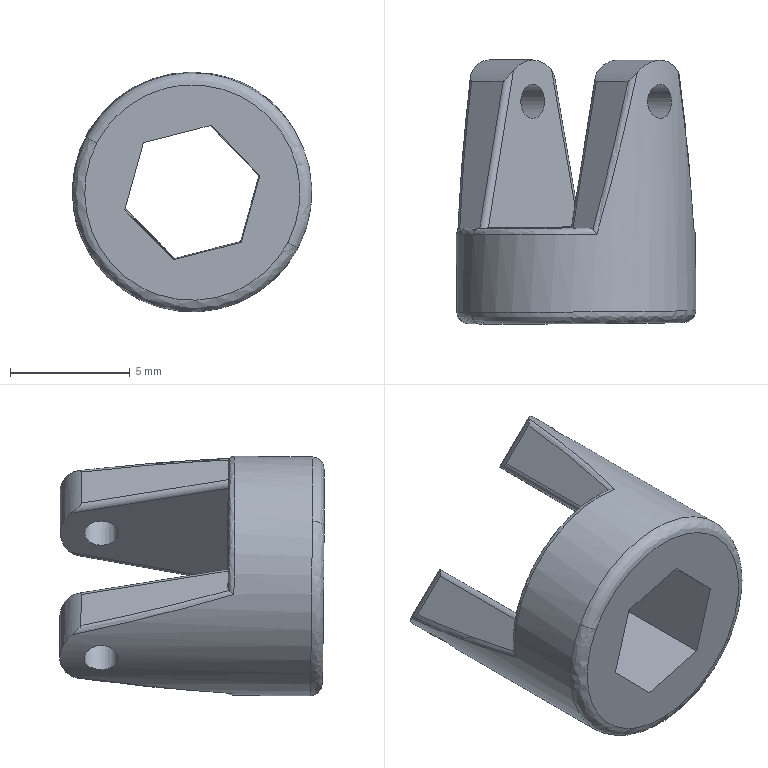Part | STEP file | Wytnij-wyci_gni_cie1_8 | 1 solid | 34 faces | box 10.019 x 11.057 x 10.028 mm | volume 351.853 mm3 | plane 17 | cylinder 9 | spline 8 | commonest cylinder face diameters 0.5 x4 1.42 x2 3.456 x2 10 x1